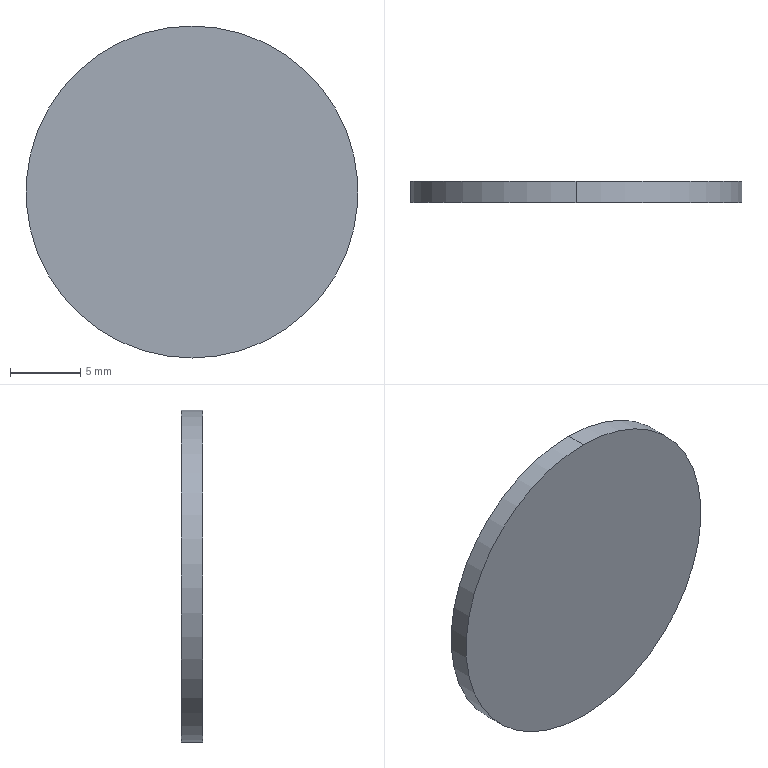Part | SolidWorks | features Extrusion 1 | 1 solid | 4 faces | box 23.6 x 1.5 x 23.6 mm | volume 656.153 mm3 | cylinder 2 | plane 2 | commonest cylinder face diameters 23.6 x2
STEP:
#1=CARTESIAN_POINT('',(0.,208.5,11.8));
#2=VERTEX_POINT('',#1);
#3=CARTESIAN_POINT('',(0.,208.5,-11.8));
#4=VERTEX_POINT('',#3);
#5=CARTESIAN_POINT('',(0.,208.5,0.));
#6=DIRECTION('',(0.,1.,0.));
#7=DIRECTION('',(0.,0.,1.));
#8=AXIS2_PLACEMENT_3D('',#5,#6,#7);
#9=CIRCLE('',#8,11.8);
#10=EDGE_CURVE('',#2,#4,#9,.T.);
#11=ORIENTED_EDGE('',*,*,#10,.T.);
#12=CARTESIAN_POINT('',(0.,210.,-11.8));
#13=VERTEX_POINT('',#12);
#14=CARTESIAN_POINT('',(0.,208.5,-11.8));
#15=DIRECTION('',(0.,1.,0.));
#16=VECTOR('',#15,1000.);
#17=LINE('',#14,#16);
#18=EDGE_CURVE('',#4,#13,#17,.T.);
#19=ORIENTED_EDGE('',*,*,#18,.T.);
#20=CARTESIAN_POINT('',(0.,210.,11.8));
#21=VERTEX_POINT('',#20);
#22=CARTESIAN_POINT('',(0.,210.,0.));
#23=DIRECTION('',(0.,1.,0.));
#24=DIRECTION('',(0.,0.,1.));
#25=AXIS2_PLACEMENT_3D('',#22,#23,#24);
#26=CIRCLE('',#25,11.8);
#27=EDGE_CURVE('',#21,#13,#26,.T.);
#28=ORIENTED_EDGE('',*,*,#27,.F.);
#29=CARTESIAN_POINT('',(0.,208.5,11.8));
#30=DIRECTION('',(0.,1.,0.));
#31=VECTOR('',#30,1000.);
#32=LINE('',#29,#31);
#33=EDGE_CURVE('',#2,#21,#32,.T.);
#34=ORIENTED_EDGE('',*,*,#33,.F.);
#35=EDGE_LOOP('',(#11,#19,#28,#34));
#36=FACE_OUTER_BOUND('',#35,.T.);
#37=CARTESIAN_POINT('',(0.,208.5,0.));
#38=DIRECTION('',(0.,1.,0.));
#39=DIRECTION('',(0.,0.,1.));
#40=AXIS2_PLACEMENT_3D('',#37,#38,#39);
#41=CYLINDRICAL_SURFACE('',#40,11.8);
#42=ADVANCED_FACE('',(#36),#41,.T.);
#43=ORIENTED_EDGE('',*,*,#18,.F.);
#44=CARTESIAN_POINT('',(0.,208.5,0.));
#45=DIRECTION('',(0.,1.,0.));
#46=DIRECTION('',(0.,0.,1.));
#47=AXIS2_PLACEMENT_3D('',#44,#45,#46);
#48=CIRCLE('',#47,11.8);
#49=EDGE_CURVE('',#4,#2,#48,.T.);
#50=ORIENTED_EDGE('',*,*,#49,.T.);
#51=ORIENTED_EDGE('',*,*,#33,.T.);
#52=CARTESIAN_POINT('',(0.,210.,0.));
#53=DIRECTION('',(0.,1.,0.));
#54=DIRECTION('',(0.,0.,1.));
#55=AXIS2_PLACEMENT_3D('',#52,#53,#54);
#56=CIRCLE('',#55,11.8);
#57=EDGE_CURVE('',#13,#21,#56,.T.);
#58=ORIENTED_EDGE('',*,*,#57,.F.);
#59=EDGE_LOOP('',(#43,#50,#51,#58));
#60=FACE_OUTER_BOUND('',#59,.T.);
#61=CARTESIAN_POINT('',(0.,208.5,0.));
#62=DIRECTION('',(0.,1.,0.));
#63=DIRECTION('',(0.,0.,1.));
#64=AXIS2_PLACEMENT_3D('',#61,#62,#63);
#65=CYLINDRICAL_SURFACE('',#64,11.8);
#66=ADVANCED_FACE('',(#60),#65,.T.);
#67=ORIENTED_EDGE('',*,*,#10,.F.);
#68=ORIENTED_EDGE('',*,*,#49,.F.);
#69=EDGE_LOOP('',(#67,#68));
#70=FACE_OUTER_BOUND('',#69,.T.);
#71=CARTESIAN_POINT('',(0.,208.5,0.));
#72=DIRECTION('',(0.,1.,0.));
#73=DIRECTION('',(0.,0.,1.));
#74=AXIS2_PLACEMENT_3D('',#71,#72,#73);
#75=PLANE('',#74);
#76=ADVANCED_FACE('',(#70),#75,.F.);
#77=ORIENTED_EDGE('',*,*,#27,.T.);
#78=ORIENTED_EDGE('',*,*,#57,.T.);
#79=EDGE_LOOP('',(#77,#78));
#80=FACE_OUTER_BOUND('',#79,.T.);
#81=CARTESIAN_POINT('',(0.,210.,0.));
#82=DIRECTION('',(0.,1.,0.));
#83=DIRECTION('',(0.,0.,1.));
#84=AXIS2_PLACEMENT_3D('',#81,#82,#83);
#85=PLANE('',#84);
#86=ADVANCED_FACE('',(#80),#85,.T.);
#87=CLOSED_SHELL('',(#42,#66,#76,#86));
#88=MANIFOLD_SOLID_BREP('',#87);
#89=CARTESIAN_POINT('',(0.,0.,0.));
#90=DIRECTION('',(0.,0.,1.));
#91=DIRECTION('',(1.,0.,0.));
#92=AXIS2_PLACEMENT_3D('',#89,#90,#91);
#93=(LENGTH_UNIT()NAMED_UNIT(*)SI_UNIT(.MILLI.,.METRE.));
#94=UNCERTAINTY_MEASURE_WITH_UNIT(LENGTH_MEASURE(0.00001),#93,'','');
#95=(NAMED_UNIT(*)PLANE_ANGLE_UNIT()SI_UNIT($,.RADIAN.));
#96=(NAMED_UNIT(*)SI_UNIT($,.STERADIAN.)SOLID_ANGLE_UNIT());
#97=(GEOMETRIC_REPRESENTATION_CONTEXT(3)GLOBAL_UNCERTAINTY_ASSIGNED_CONTEXT((#94))GLOBAL_UNIT_ASSIGNED_CONTEXT((#93,#95,#96))REPRESENTATION_CONTEXT('',''));
#98=ADVANCED_BREP_SHAPE_REPRESENTATION('',(#88,#92),#97);